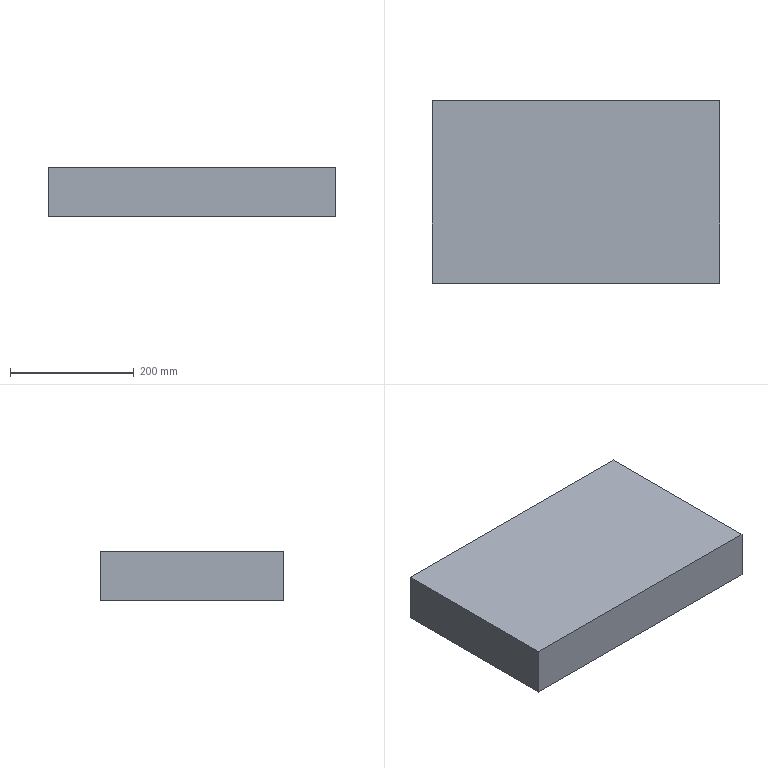Part | SolidWorks | features Extrusion 1 | 1 solid | 6 faces | box 465 x 295 x 80 mm | volume 10974000 mm3 | plane 6
STEP:
#1=CARTESIAN_POINT('',(232.5,-147.5,0.));
#2=VERTEX_POINT('',#1);
#3=CARTESIAN_POINT('',(232.5,147.5,0.));
#4=VERTEX_POINT('',#3);
#5=CARTESIAN_POINT('',(232.5,-147.5,0.));
#6=DIRECTION('',(0.,1.,0.));
#7=VECTOR('',#6,1000.);
#8=LINE('',#5,#7);
#9=EDGE_CURVE('',#2,#4,#8,.T.);
#10=ORIENTED_EDGE('',*,*,#9,.T.);
#11=CARTESIAN_POINT('',(232.5,147.5,80.));
#12=VERTEX_POINT('',#11);
#13=CARTESIAN_POINT('',(232.5,147.5,80.));
#14=DIRECTION('',(0.,0.,-1.));
#15=VECTOR('',#14,1000.);
#16=LINE('',#13,#15);
#17=EDGE_CURVE('',#12,#4,#16,.T.);
#18=ORIENTED_EDGE('',*,*,#17,.F.);
#19=CARTESIAN_POINT('',(232.5,-147.5,80.));
#20=VERTEX_POINT('',#19);
#21=CARTESIAN_POINT('',(232.5,-147.5,80.));
#22=DIRECTION('',(0.,1.,0.));
#23=VECTOR('',#22,1000.);
#24=LINE('',#21,#23);
#25=EDGE_CURVE('',#20,#12,#24,.T.);
#26=ORIENTED_EDGE('',*,*,#25,.F.);
#27=CARTESIAN_POINT('',(232.5,-147.5,80.));
#28=DIRECTION('',(0.,0.,-1.));
#29=VECTOR('',#28,1000.);
#30=LINE('',#27,#29);
#31=EDGE_CURVE('',#20,#2,#30,.T.);
#32=ORIENTED_EDGE('',*,*,#31,.T.);
#33=EDGE_LOOP('',(#10,#18,#26,#32));
#34=FACE_OUTER_BOUND('',#33,.T.);
#35=CARTESIAN_POINT('',(232.5,-147.5,80.));
#36=DIRECTION('',(-1.,0.,0.));
#37=DIRECTION('',(0.,0.,1.));
#38=AXIS2_PLACEMENT_3D('',#35,#36,#37);
#39=PLANE('',#38);
#40=ADVANCED_FACE('',(#34),#39,.F.);
#41=CARTESIAN_POINT('',(-232.5,147.5,0.));
#42=VERTEX_POINT('',#41);
#43=CARTESIAN_POINT('',(-232.5,147.5,0.));
#44=DIRECTION('',(-1.,0.,0.));
#45=VECTOR('',#44,1000.);
#46=LINE('',#43,#45);
#47=EDGE_CURVE('',#4,#42,#46,.T.);
#48=ORIENTED_EDGE('',*,*,#47,.T.);
#49=CARTESIAN_POINT('',(-232.5,147.5,80.));
#50=VERTEX_POINT('',#49);
#51=CARTESIAN_POINT('',(-232.5,147.5,80.));
#52=DIRECTION('',(0.,0.,-1.));
#53=VECTOR('',#52,1000.);
#54=LINE('',#51,#53);
#55=EDGE_CURVE('',#50,#42,#54,.T.);
#56=ORIENTED_EDGE('',*,*,#55,.F.);
#57=CARTESIAN_POINT('',(-232.5,147.5,80.));
#58=DIRECTION('',(-1.,0.,0.));
#59=VECTOR('',#58,1000.);
#60=LINE('',#57,#59);
#61=EDGE_CURVE('',#12,#50,#60,.T.);
#62=ORIENTED_EDGE('',*,*,#61,.F.);
#63=ORIENTED_EDGE('',*,*,#17,.T.);
#64=EDGE_LOOP('',(#48,#56,#62,#63));
#65=FACE_OUTER_BOUND('',#64,.T.);
#66=CARTESIAN_POINT('',(-232.5,147.5,80.));
#67=DIRECTION('',(0.,-1.,0.));
#68=DIRECTION('',(0.,0.,-1.));
#69=AXIS2_PLACEMENT_3D('',#66,#67,#68);
#70=PLANE('',#69);
#71=ADVANCED_FACE('',(#65),#70,.F.);
#72=CARTESIAN_POINT('',(-232.5,-147.5,0.));
#73=VERTEX_POINT('',#72);
#74=CARTESIAN_POINT('',(-232.5,-147.5,0.));
#75=DIRECTION('',(0.,-1.,0.));
#76=VECTOR('',#75,1000.);
#77=LINE('',#74,#76);
#78=EDGE_CURVE('',#42,#73,#77,.T.);
#79=ORIENTED_EDGE('',*,*,#78,.T.);
#80=CARTESIAN_POINT('',(-232.5,-147.5,80.));
#81=VERTEX_POINT('',#80);
#82=CARTESIAN_POINT('',(-232.5,-147.5,80.));
#83=DIRECTION('',(0.,0.,-1.));
#84=VECTOR('',#83,1000.);
#85=LINE('',#82,#84);
#86=EDGE_CURVE('',#81,#73,#85,.T.);
#87=ORIENTED_EDGE('',*,*,#86,.F.);
#88=CARTESIAN_POINT('',(-232.5,-147.5,80.));
#89=DIRECTION('',(0.,-1.,0.));
#90=VECTOR('',#89,1000.);
#91=LINE('',#88,#90);
#92=EDGE_CURVE('',#50,#81,#91,.T.);
#93=ORIENTED_EDGE('',*,*,#92,.F.);
#94=ORIENTED_EDGE('',*,*,#55,.T.);
#95=EDGE_LOOP('',(#79,#87,#93,#94));
#96=FACE_OUTER_BOUND('',#95,.T.);
#97=CARTESIAN_POINT('',(-232.5,-147.5,80.));
#98=DIRECTION('',(1.,0.,0.));
#99=DIRECTION('',(0.,0.,-1.));
#100=AXIS2_PLACEMENT_3D('',#97,#98,#99);
#101=PLANE('',#100);
#102=ADVANCED_FACE('',(#96),#101,.F.);
#103=CARTESIAN_POINT('',(-232.5,-147.5,0.));
#104=DIRECTION('',(1.,0.,0.));
#105=VECTOR('',#104,1000.);
#106=LINE('',#103,#105);
#107=EDGE_CURVE('',#73,#2,#106,.T.);
#108=ORIENTED_EDGE('',*,*,#107,.T.);
#109=ORIENTED_EDGE('',*,*,#31,.F.);
#110=CARTESIAN_POINT('',(-232.5,-147.5,80.));
#111=DIRECTION('',(1.,0.,0.));
#112=VECTOR('',#111,1000.);
#113=LINE('',#110,#112);
#114=EDGE_CURVE('',#81,#20,#113,.T.);
#115=ORIENTED_EDGE('',*,*,#114,.F.);
#116=ORIENTED_EDGE('',*,*,#86,.T.);
#117=EDGE_LOOP('',(#108,#109,#115,#116));
#118=FACE_OUTER_BOUND('',#117,.T.);
#119=CARTESIAN_POINT('',(-232.5,-147.5,80.));
#120=DIRECTION('',(0.,1.,0.));
#121=DIRECTION('',(0.,0.,1.));
#122=AXIS2_PLACEMENT_3D('',#119,#120,#121);
#123=PLANE('',#122);
#124=ADVANCED_FACE('',(#118),#123,.F.);
#125=ORIENTED_EDGE('',*,*,#25,.T.);
#126=ORIENTED_EDGE('',*,*,#61,.T.);
#127=ORIENTED_EDGE('',*,*,#92,.T.);
#128=ORIENTED_EDGE('',*,*,#114,.T.);
#129=EDGE_LOOP('',(#125,#126,#127,#128));
#130=FACE_OUTER_BOUND('',#129,.T.);
#131=CARTESIAN_POINT('',(0.,0.,80.));
#132=DIRECTION('',(0.,0.,-1.));
#133=DIRECTION('',(-1.,0.,0.));
#134=AXIS2_PLACEMENT_3D('',#131,#132,#133);
#135=PLANE('',#134);
#136=ADVANCED_FACE('',(#130),#135,.F.);
#137=ORIENTED_EDGE('',*,*,#9,.F.);
#138=ORIENTED_EDGE('',*,*,#107,.F.);
#139=ORIENTED_EDGE('',*,*,#78,.F.);
#140=ORIENTED_EDGE('',*,*,#47,.F.);
#141=EDGE_LOOP('',(#137,#138,#139,#140));
#142=FACE_OUTER_BOUND('',#141,.T.);
#143=CARTESIAN_POINT('',(0.,0.,0.));
#144=DIRECTION('',(0.,0.,-1.));
#145=DIRECTION('',(-1.,0.,0.));
#146=AXIS2_PLACEMENT_3D('',#143,#144,#145);
#147=PLANE('',#146);
#148=ADVANCED_FACE('',(#142),#147,.T.);
#149=CLOSED_SHELL('',(#40,#71,#102,#124,#136,#148));
#150=MANIFOLD_SOLID_BREP('',#149);
#151=CARTESIAN_POINT('',(0.,0.,0.));
#152=DIRECTION('',(0.,0.,1.));
#153=DIRECTION('',(1.,0.,0.));
#154=AXIS2_PLACEMENT_3D('',#151,#152,#153);
#155=(LENGTH_UNIT()NAMED_UNIT(*)SI_UNIT(.MILLI.,.METRE.));
#156=UNCERTAINTY_MEASURE_WITH_UNIT(LENGTH_MEASURE(0.00001),#155,'','');
#157=(NAMED_UNIT(*)PLANE_ANGLE_UNIT()SI_UNIT($,.RADIAN.));
#158=(NAMED_UNIT(*)SI_UNIT($,.STERADIAN.)SOLID_ANGLE_UNIT());
#159=(GEOMETRIC_REPRESENTATION_CONTEXT(3)GLOBAL_UNCERTAINTY_ASSIGNED_CONTEXT((#156))GLOBAL_UNIT_ASSIGNED_CONTEXT((#155,#157,#158))REPRESENTATION_CONTEXT('',''));
#160=ADVANCED_BREP_SHAPE_REPRESENTATION('',(#150,#154),#159);